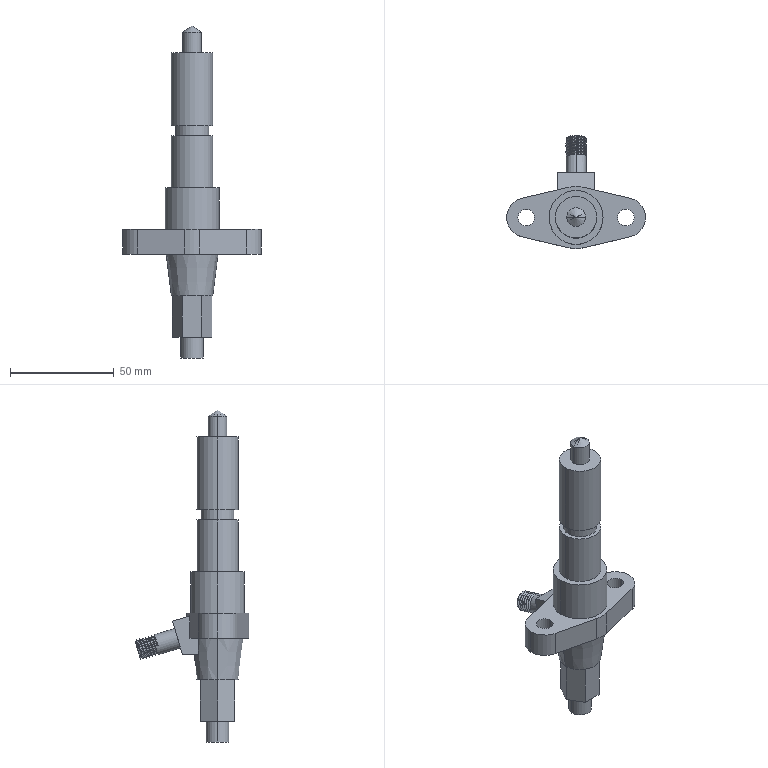Part | SolidWorks | features BaseBody 6 | 6 solids | 88 faces | box 67 x 54.595 x 160 mm | volume 65143 mm3 | cylinder 49 | plane 33 | cone 4 | spline 2 | commonest cylinder face diameters 8.25 x14 9.75 x14 8 x4 20 x4 19 x3 9 x2